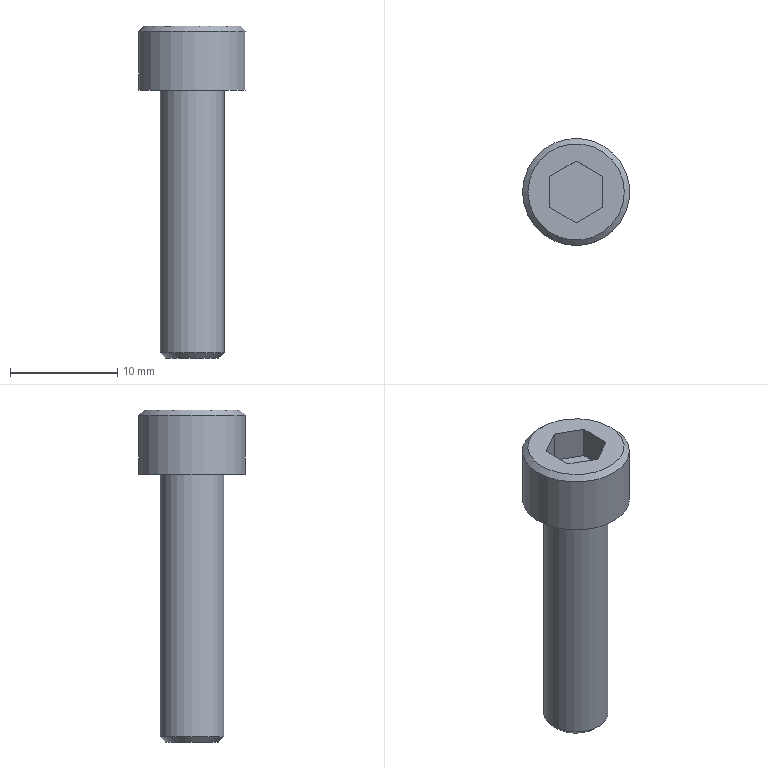Part | STEP file | solid 101 | 1 solid | 14 faces | box 10 x 10 x 31 mm | volume 1107 mm3 | plane 10 | cylinder 2 | cone 2 | commonest cylinder face diameters 6 x1 10 x1